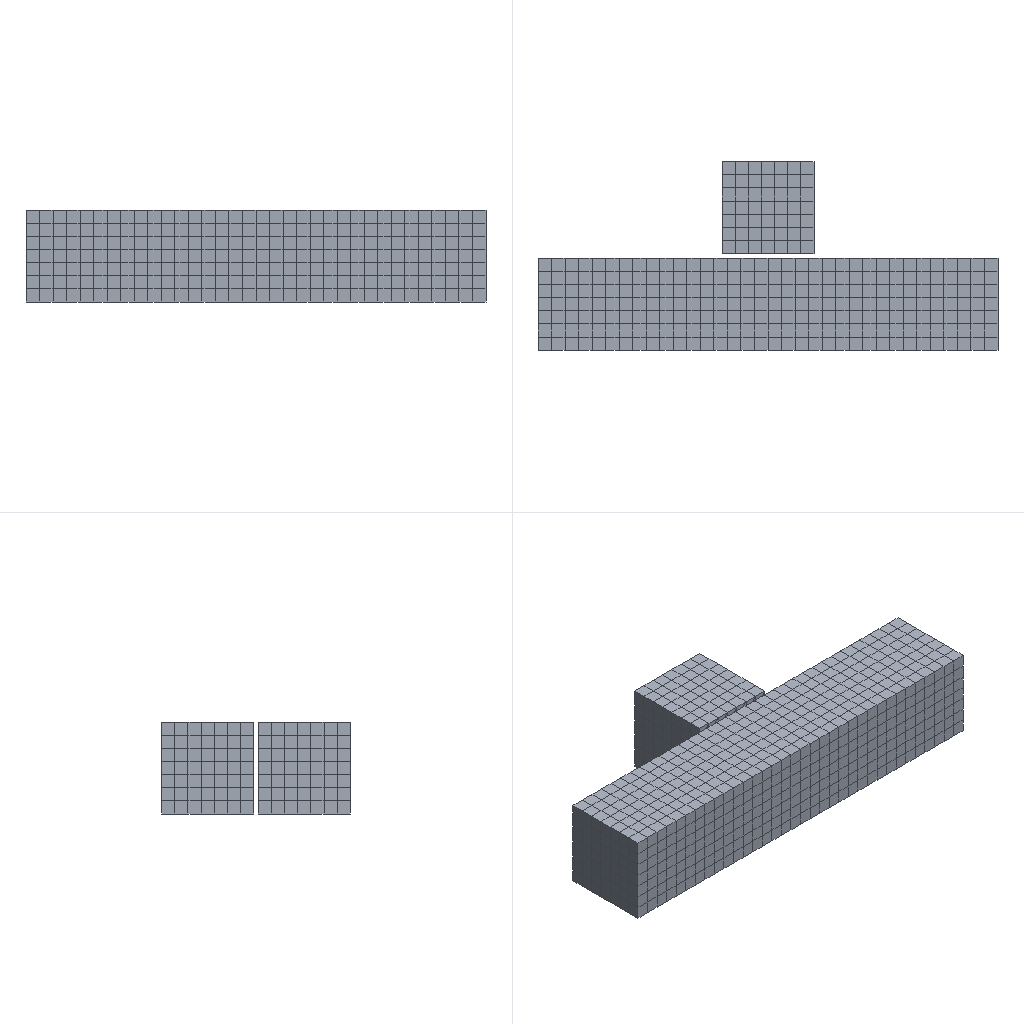Simulation study | ansys workbench
Ansys APDL input file, long lists of numbers shortened:
/batch
/config,noeldb,1     ! force off writing results to database
*get,_wallstrt,active,,time,wall
! ANSYS input file written by Workbench version 2023 R1
! File used for geometry attach:
/title,E1.7.2--Static Structural (A5)
! ****** Begin Custom Load Command Snippet ******
/COM, ACT Extensions:
/COM,     LSDYNA, 2023.1
/COM,/COM,     ANSYSMotion, 2023.1
/COM,
! ****** End   Custom Load Command Snippet ******
*DIM,_wb_ProjectScratch_dir,string,248
_wb_ProjectScratch_dir(1) = ''
*DIM,_wb_SolverFiles_dir,string,248
_wb_SolverFiles_dir(1) = ''
*DIM,_wb_userfiles_dir,string,248
_wb_userfiles_dir(1) = ''
/com,--- Data in consistent NMM units. See Solving Units in the help system for more information.
/units,MPA
/nopr
/wb,file,start              !  signify a WB generated input file
/prep7
! Turn off shape checking because checks already performed inside WB mesher.
! See help system for more information.
SHPP,OFF,,NOWARN
/nolist
etcon,set             ! allow ANSYS to choose best KEYOP's for 180x elements, resets any applicable keyopt to MAPDL defaults
/com,*********** Nodes for the whole assembly ***********
nblock,3,,11211
(1i9,3e20.9e3)
        1     2.857142857E+04     1.928571429E+03     1.428571429E+03
! (10191 more lines like these left out)
-1
/wb,elem,start            !  set before creation of elements
/com,*********** Elements for Body 1 "1" ***********
et,1,186
keyo,1,2,1          ! set full integration on SOLID186
eblock,19,solid,,1666
(19i9)
        1        1        1        1        0        0        0        0       20        0      344     1857     3898     3566     3528     3242     4096     3565     3559
! (3331 more lines like these left out)
-1
/com,*********** Elements for Body 2 "2" ***********
et,2,186
keyo,2,2,1          ! set full integration on SOLID186
eblock,19,solid,,343
(19i9)
        2        2        2        2        0        0        0        0       20        0        1        1      452      465      471      252      463      464      507
! (685 more lines like these left out)
-1
/wb,elem,end               !  done creating elements
/com,*********** Send User Defined Coordinate System(s) ***********
csys,0
toffst,273.15,  ! Temperature offset from absolute zero
/com,*********** Set Reference Temperature ***********
tref,22.
/wb,mat,start              !  starting to send materials
/com,*********** Send Materials ***********
Temperature = 'TEMP' ! Temperature
MP,DENS,1,7.85e-09,	! tonne mm^-3
MP,ALPX,1,1.2e-05,	! C^-1
MP,C,1,434000000,	! mm^2 s^-2 C^-1
MP,KXX,1,60.5,	! tonne mm s^-3 C^-1
MP,RSVX,1,0.00017,	! ohm mm
MP,EX,1,200000,	! tonne s^-2 mm^-1
MP,NUXY,1,0.3,
MP,MURX,1,10000,
Temperature = 'TEMP' ! Temperature
MP,DENS,2,7.85e-09,	! tonne mm^-3
MP,ALPX,2,1.2e-05,	! C^-1
MP,C,2,434000000,	! mm^2 s^-2 C^-1
MP,KXX,2,60.5,	! tonne mm s^-3 C^-1
MP,RSVX,2,0.00017,	! ohm mm
MP,EX,2,200000,	! tonne s^-2 mm^-1
MP,NUXY,2,0.3,
MP,MURX,2,10000,
/wb,mat,end                !  done sending materials
!************************* Model Summary ********************
!1,	Structural Steel,	matid,	1
!2,	Structural Steel,	matid,	2
!************************* End Model Summary ********************
! get the diagonal of the bounding box. Needed later for other things
*get,_xmin,node,,mnloc,x
*get,_ymin,node,,mnloc,y
*get,_zmin,node,,mnloc,z
*get,_xmax,node,,mxloc,x
*get,_ymax,node,,mxloc,y
*get,_zmax,node,,mxloc,z
_ASMDIAG=(_xmax-_xmin)*(_xmax-_xmin)+(_ymax-_ymin)*(_ymax-_ymin)+(_zmax-_zmin)*(_zmax-_zmin)
_ASMDIAG=SQRT(_ASMDIAG)
/wb,contact,start          !  starting to send contact
/com,*********** Create Contact "Frictional - 2 To 1" ***********
/com,            Real Constant Set For Above Contact Is 4 & 3
*set,tid,4
*set,cid,3
r,tid
r,cid
et,tid,170
et,cid,174
eblock,10,,,49
(15i9)
     3354        4        4        4        0      465      471      507      464     1776     1788     1774     1773
! (48 more lines like these left out)
-1
eblock,10,,,49
(15i9)
     3403        3        3        3        0      465      471      507      464     1776     1788     1774     1773
! (48 more lines like these left out)
-1
eblock,10,,,238
(15i9)
     3452        3        4        3        0     3514     3579     3578     3515     9111     9237     9113     9110
! (237 more lines like these left out)
-1
eblock,10,,,238
(15i9)
     3690        4        3        4        0     3514     3579     3578     3515     9111     9237     9113     9110
! (237 more lines like these left out)
-1
keyo,cid,8,2               ! auto create asymmetric contact (from Program Controlled setting)
keyo,cid,10,0              ! adjust contact stiffness each NR iteration
keyo,cid,12,0              ! standard contact
mp,mu,cid,0.15      ! unitless
keyo,cid,18,0              ! finite small sliding
keyo,cid,2,0               ! augmented Lagrange (from Program Controlled setting)
keyo,cid,4,0               ! on Gauss point (from Program Controlled setting)
keyo,cid,9,1               ! ignore initial gaps/penetration
keyo,cid,5,1               ! auto CNOF adjustment to close geometric gap only
keyo,cid,7,1               ! Automatic Bisection
rmod,tid,3,1.       ! FKN
rmod,tid,5,0.       ! ICONT
rmod,tid,6,0.       ! PINB
rmod,tid,10,0.      ! CNOF
rmod,tid,12,0.      ! FKT
rmod,tid,36,33      ! WB DSID
rmod,cid,3,1.       ! FKN
rmod,cid,5,0.       ! ICONT
rmod,cid,6,0.       ! PINB
rmod,cid,10,0.      ! CNOF
rmod,cid,12,0.      ! FKT
rmod,cid,36,33      ! WB DSID
nsel,all
esel,all
/wb,contact,end            !  done creating contacts
/golist
/wb,load,start             !  starting to send loads
/com,*********** Fixed Supports ***********
CMBLOCK,_FIXEDSU,NODE,      352
(8i10)
      3474      3475      3476      3477      3478      3479      3480      3481
! (43 more lines like these left out)
cmsel,s,_FIXEDSU
d,all,all
nsel,all
/com,*********** Define Pressure Vector Using Surface Effect Elements ***********
local,12,0,0.,0.,0.,0.,0.,0.
csys,0
et,5,154
mat,5
eblock,10,,,49
(15i9)
     3928        5        5        5       12      421      373      303      302     1606     1467     1464     1465
! (48 more lines like these left out)
-1
esel,s,type,,5
keyop,5,2,1                ! Apply load in local coordinate system
keyop,5,7,0                ! Use deformed area for application of load
esel,all
/gst,on,on
fini
*get,_numnode,node,0,count
*get,_numelem,elem,0,count
*get, _MAXELEMNUM, elem, 0, NUM, MAX
*get, _MAXNODENUM, node, 0, NUM, MAX
*get, _MAXELEMTYPE, etyp, 0, NUM, MAX
*get, _MAXREALCONST, rcon, 0, NUM, MAX
/go
/wb,load,end               !  done creating loads
/com,--- Number of total nodes = %_numnode%
/com,--- Number of contact elements = 623
/com,--- Number of spring elements = 0
/com,--- Number of bearing elements = 0
/com,--- Number of solid elements = 2009
/com,--- Number of condensed parts = 0
/com,--- Number of total elements = %_numelem%
*get,_wallbsol,active,,time,wall
/com,****************************************************************************
/com,*************************    SOLUTION       ********************************
/com,****************************************************************************
/solu
antype,0                   ! static analysis
_thickRatio=  1     ! Ratio of thick parts in the model
eqsl,pcg,1e-8,,,,,,1
cntr,print,1               ! print out contact info and also make no initial contact an error
nldiag,cont,iter           ! print out contact info each equilibrium iteration
rescontrol,define,last,last,,dele	   ! Program Controlled
/com,****************************************************
/com,******************* SOLVE FOR LS 1 OF 1 ****************
esel,s,type,,5
nsle
sfe,all,1,pres,1,0.
sfe,all,2,pres,1,-1.
sfe,all,3,pres,1,0.
nsel,all
esel,all
/nopr
/gopr
autots,on                  ! Workbench Program Controlled automatic time stepping
nsub,1,10,1                ! due to presence of general nonlinear
time,1.
outres,erase
outres,all,none
outres,nsol,all,
outres,rsol,all
outres,eangl,all
outres,etmp,all
outres,veng,all
outres,strs,all,
outres,epel,all,
outres,eppl,all,
outres,cont,all,
! *********** WB SOLVE COMMAND ***********
! check interactive state
*get,ANSINTER_,active,,int
*if,ANSINTER_,ne,0,then
/eof
*endif
solve
/com *************** Write FE CONNECTORS *********
CEWRITE,file,ce,,INTE
/com,****************************************************
/com,*************** FINISHED SOLVE FOR LS 1 *************
*get,_wallasol,active,,time,wall
/nopr
*get,_numnode,node,0,count
*get,_numelem,elem,0,count
*get, _MAXELEMNUM, elem, 0, NUM, MAX
*get, _MAXNODENUM, node, 0, NUM, MAX,,,INTERNAL
*get, _MAXELEMTYPE, etyp, 0, NUM, MAX
*get, _MAXREALCONST, rcon, 0, NUM, MAX
*get,_NSOLTHREADS,active,0,ntfs
*get,_NSOLPROCESSES,active,0,npfs
/gopr
*get,_PCGITER,active,,solu,cgiter
/post1
xmlo,ENCODING,ISO-8859-1
xmlo,parm
/xml,parm,xml
fini
/gopr
*get,_walldone,active,,time,wall
_preptime=(_wallbsol-_wallstrt)*3600
_solvtime=(_wallasol-_wallbsol)*3600
_posttime=(_walldone-_wallasol)*3600
_totaltim=(_walldone-_wallstrt)*3600
*get,_dlbratio,active,0,solu,dlbr
*get,_combtime,active,0,solu,comb
*get,_ssmode,active,0,solu,ssmm
*get,_ndofs,active,0,solu,ndof
/com,--- Total number of nodes = %_numnode%
/com,--- Total number of elements = %_numelem%
/com,--- Element load balance ratio = %_dlbratio%
/com,--- Time to combine distributed files = %_combtime%
/com,--- Sparse memory mode = %_ssmode%
/com,--- Number of DOF = %_ndofs%
/wb,file,end               ! done with WB generated input